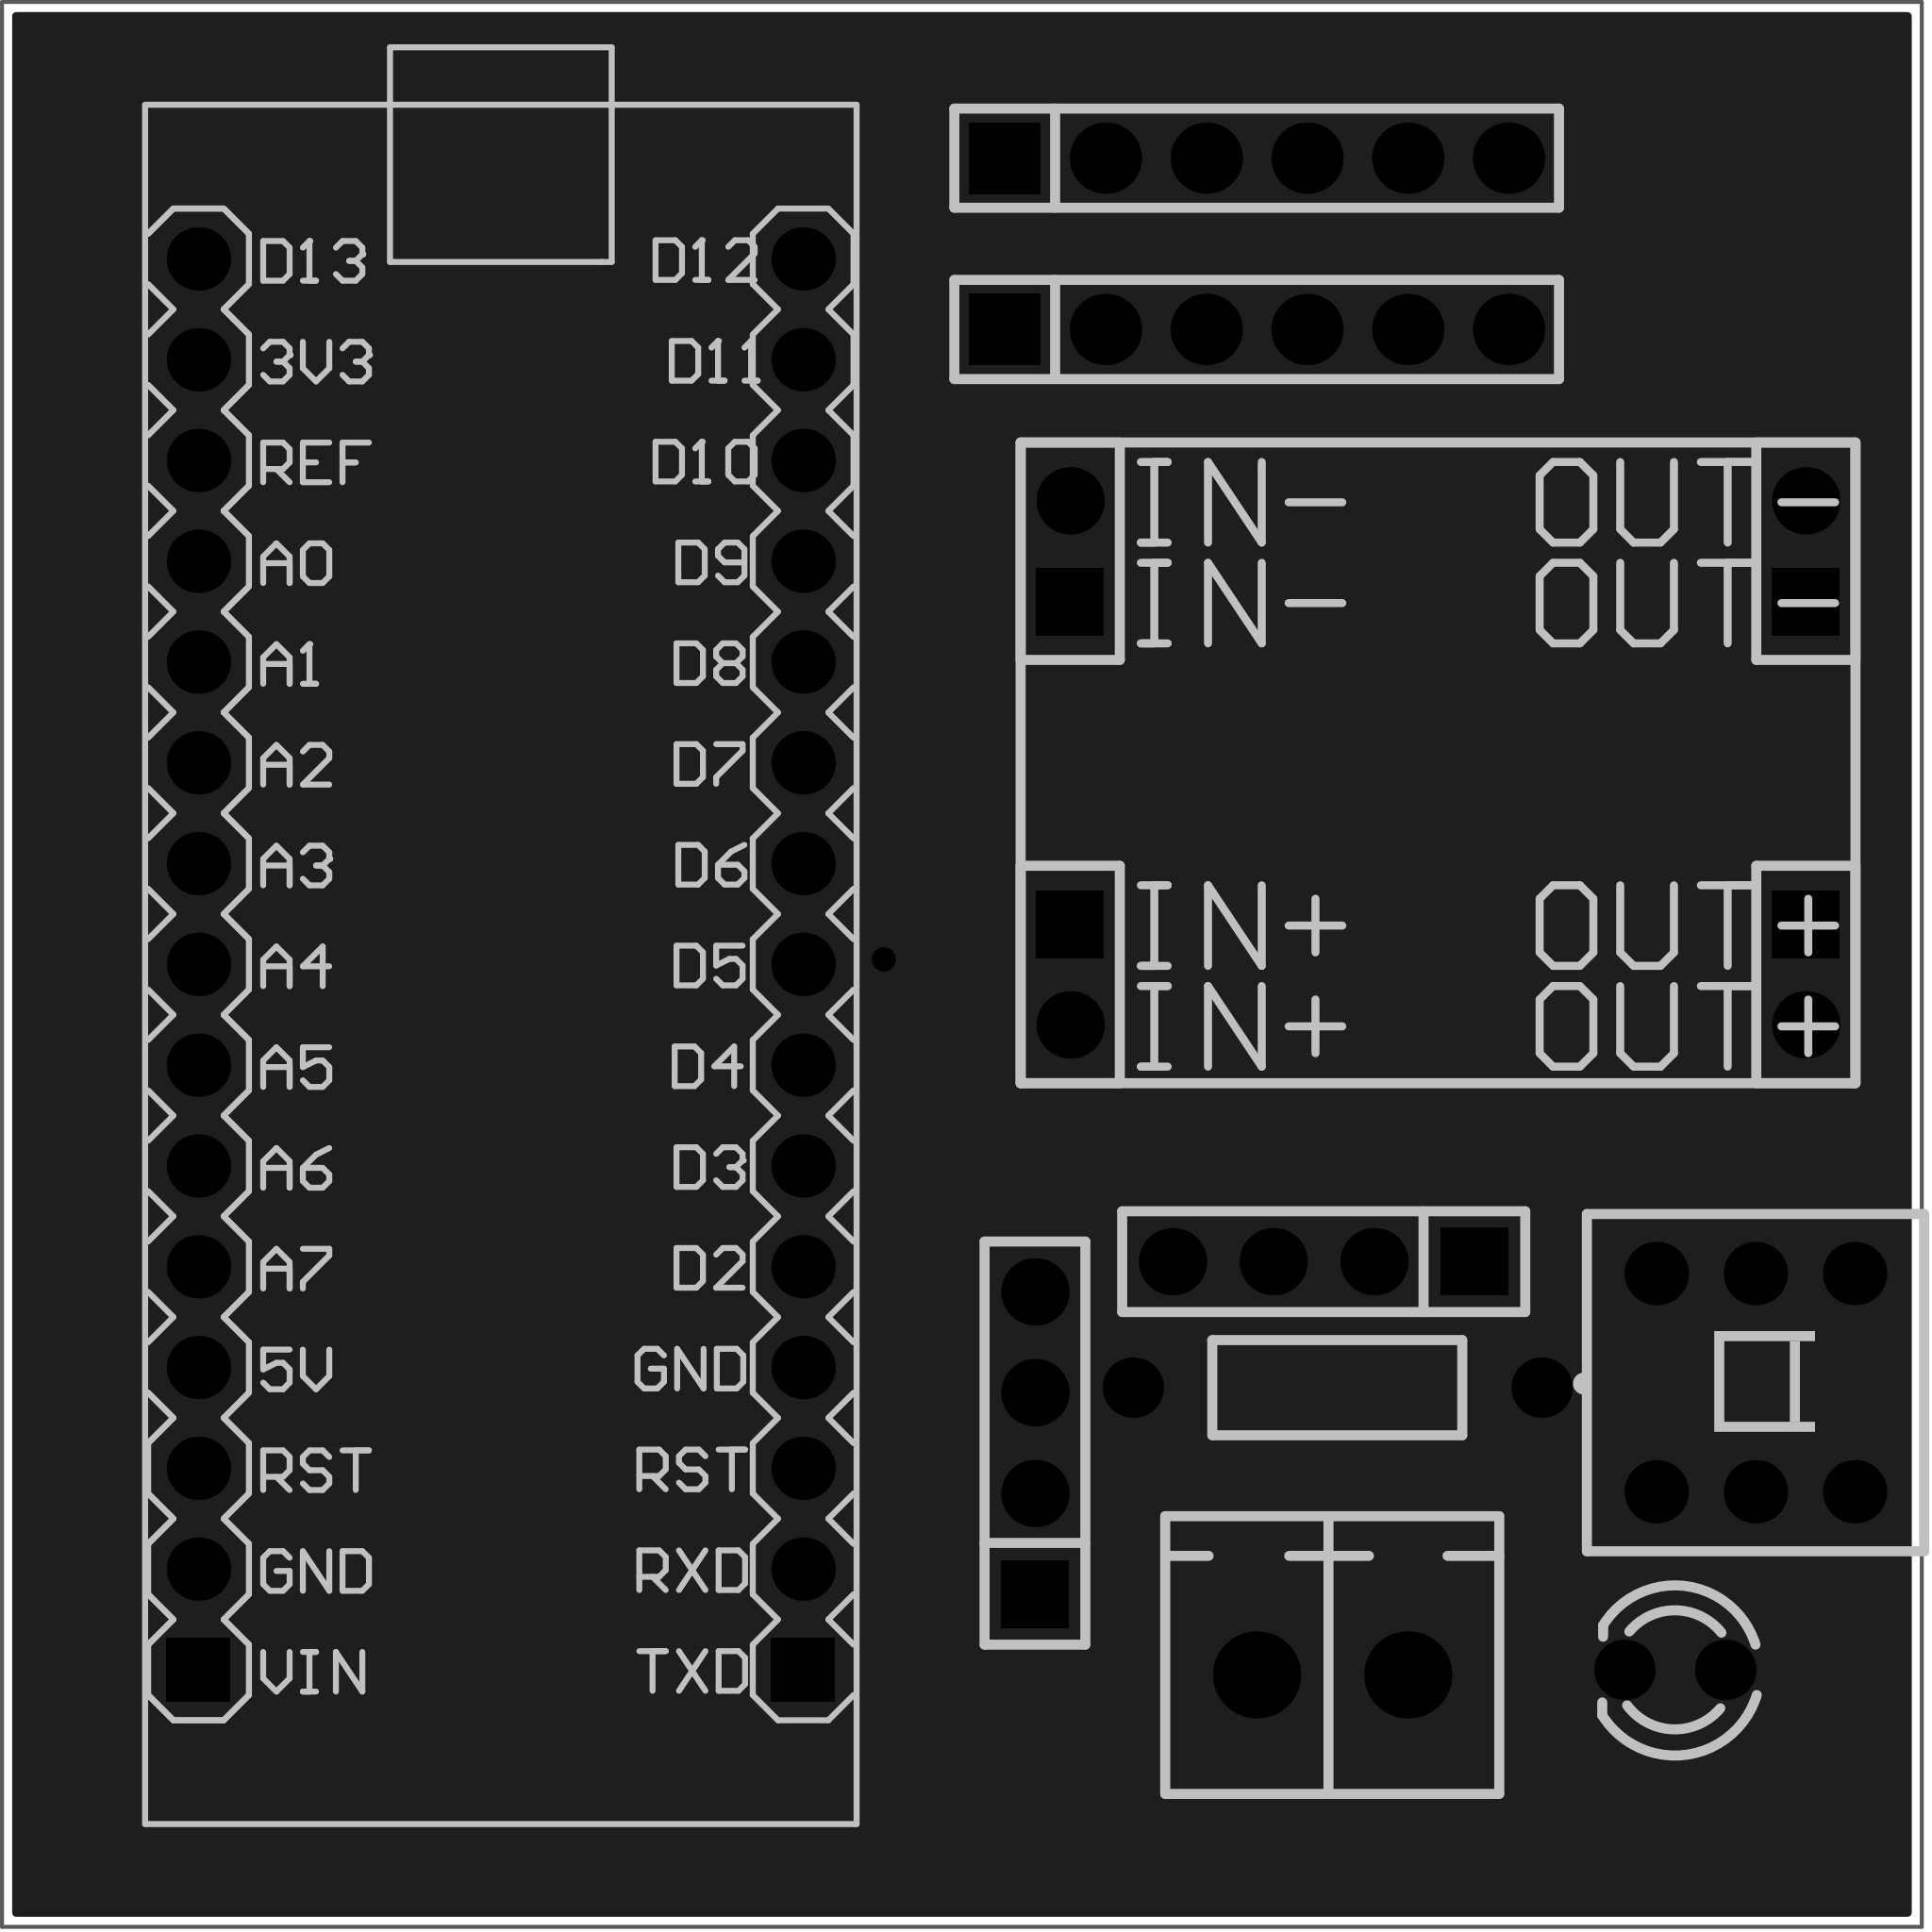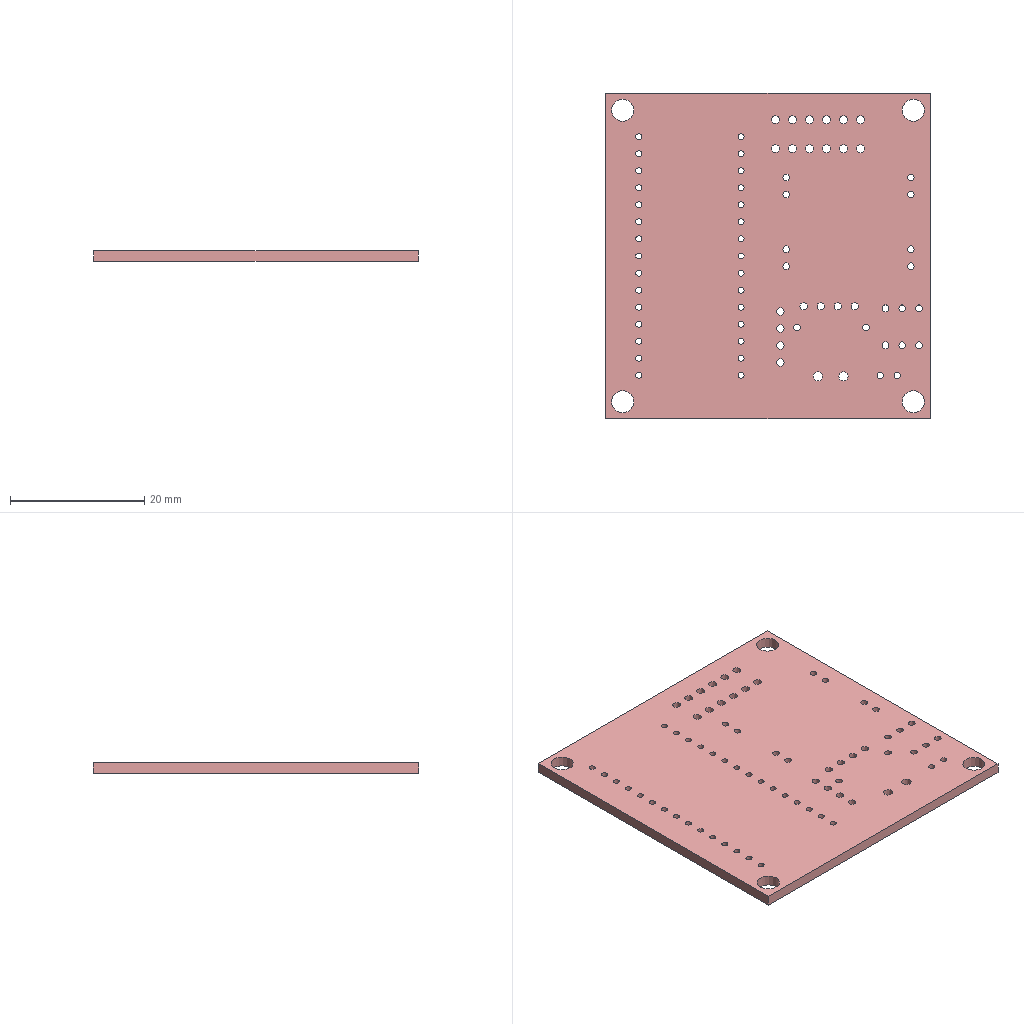Circuit board layout | Altium Designer | box 48.4 x 48.5 x 1.6 mm
Layer stack:
# Altium Designer layer stack of  (unit mm; dielectric type: 0 none, 1 core, 2 prepreg, 3 surface material)
index,name,kind,layer,copper_thickness_mm,dielectric_type,dielectric_thickness_mm,dielectric_material,dielectric_constant
0,Top Paste Mask Layer,other,,,,,,
1,Top Silkscreen Layer,other,,,,,,
2,Top Solder Mask Layer,dielectric,,,3,0.01,,3.3
3,Top Layer,copper,Top Layer,0.035,,,,
4,Dielectric1,dielectric,,,3,1.51,FR4,4.5
5,Bottom Layer,copper,Bottom Layer,0.035,,,,
6,Bottom Solder Mask Layer,dielectric,,,3,0.01,,3.3
7,Bottom Silkscreen Layer,other,,,,,,
8,Bottom Paste Mask Layer,other,,,,,,
# drill layer pairs: low layer,high layer
drill_pair,Top Layer,Bottom Layer
Part placement:
Designator,Comment,Layer,Footprint,Center-X(mm),Center-Y(mm),Rotation
H1,,TopLayer,HDR-TH_4P-P2.54-V-M,112.307,95.378,180
H2,,TopLayer,HDR-TH_4P-P2.54-V-M,105.029,90.805,90
H3,,TopLayer,HDR-TH_8P-P2.54-V-M,115.189,107.95,0
H4,,TopLayer,HDR-TH_6P-P2.54-V-M-1,110.617,118.872,0
H5,,TopLayer,HDR-TH_6P-P2.54-V-M-1,110.617,123.19,0
KEY1,Self-locking switch,TopLayer,SW-TH_6P-L8.5-W8.5-P2.54,123.19,92.329,0
LED1,,TopLayer,LED_TH-3mm,121.158,85.09,180
R1,1kΩ,TopLayer,Res_1/4W,112.649,92.202,180
U1,2P-P3.81_KF2EDGV-3.81-2P,TopLayer,CONN-TH_2P-P3.81_KF2EDGV-3.81-2P,112.522,84.963,180
U2,ARDUINO_NANO,TopLayer,COMM-TH_ARDUINO_NANO,91.567,102.87,270
Pad and via stacks:
# Altium Designer via and pad stacks of  (unit mm). Each distinct definition once, with the count of objects using it.
# via: kind,start_layer,end_layer,hole_mm,diameter_mm,mode(0 simple;1 top-mid-bottom;2 full stack),diameter_per_layer,count,example_net
# pad: kind,layer,hole_mm,hole_type(0 round;1 square;2 slot),plating,top_size,top_shape(1 round;2 rect;3 octagon;9 rounded rect),mid_size,bottom_size,mode,footprint,size_per_layer,count,example
pad,Multi-Layer,1.1,0,plated,1.7x1.7,2,1.7x1.7,1.7x1.7,0,HDR-TH_4P-P2.54-V-M,,2,H1.1
pad,Multi-Layer,1.1,0,plated,1.7x1.7,1,1.7x1.7,1.7x1.7,0,HDR-TH_4P-P2.54-V-M,,6,H1.2
pad,Multi-Layer,1,0,plated,1.7x1.7,2,1.7x1.7,1.7x1.7,0,HDR-TH_8P-P2.54-V-M,,4,H3.2
pad,Multi-Layer,1,0,plated,1.7x1.7,1,1.7x1.7,1.7x1.7,0,HDR-TH_8P-P2.54-V-M,,4,H3.1
pad,Multi-Layer,1.2,0,plated,1.8x1.8,1,1.8x1.8,1.8x1.8,0,HDR-TH_6P-P2.54-V-M-1,,10,H4.6
pad,Multi-Layer,1.2,0,plated,1.8x1.8,2,1.8x1.8,1.8x1.8,0,HDR-TH_6P-P2.54-V-M-1,,2,H4.1
pad,Multi-Layer,1,0,plated,1.6x1.6,1,1.6x1.6,1.6x1.6,0,SW-TH_6P-L8.5-W8.5-P2.54,,6,KEY1.4
pad,Multi-Layer,0.9144,0,plated,1.524x1.524,1,1.524x1.524,1.524x1.524,0,LED_TH-3mm,,2,LED1.1
pad,Multi-Layer,1,0,plated,1.524x1.524,1,1.524x1.524,1.524x1.524,0,Res_1/4W,,2,R1.1
pad,Multi-Layer,1.4,0,plated,2.2x2.2,1,2.2x2.2,2.2x2.2,0,CONN-TH_2P-P3.81_KF2EDGV-3.81-2P,,2,U1.2
pad,Multi-Layer,0.9,0,plated,1.6x1.6,2,1.6x1.6,1.6x1.6,0,COMM-TH_ARDUINO_NANO,,2,U2.1
pad,Multi-Layer,0.9,0,plated,1.6x1.6,1,1.6x1.6,1.6x1.6,0,COMM-TH_ARDUINO_NANO,,28,U2.29
via,Top Layer,Bottom Layer,0.3048,0.61,0,,1,ECHO
Copper pours:
name,layer,net,type(0 solid;1 hatched;2 none)
Top Layer-GND,Top Layer,GND,0
Bottom Layer-GND,Bottom Layer,GND,0
Design rules, without the lines most boards share:
# Altium Designer design rules of  (exported by Altium Designer, unit mm)
# columns: name | kind | enabled | priority | scope1 | scope2 | descriptor | typed fields (field=value)
copperThickness1oz_2 | 2 | enabled | 2 | All | All | Width Constraint (Min=5mil) (Max=100mil) (Preferred=30mil) (All) |
viaSize | 11 | enabled | 1 | All | All | Routing Via (MinHoleWidth=11.811mil) (MaxHoleWidth=248.032mil) (PreferredHoleWidth=12.008mil) (MinWidth=19.685mil) (MaxWidth=393.701mil) (PreferedWidth=24.016mil) (All) | via_min_hole=0.3 via_max_hole=6.3 via_preferred_diameter=0.61 via_preferred_hole=0.305
solderMaskExpansion | 13 | enabled | 2 | All | All | Solder Mask Expansion (Expansion =2.008mil) (All) | expansion=0.051